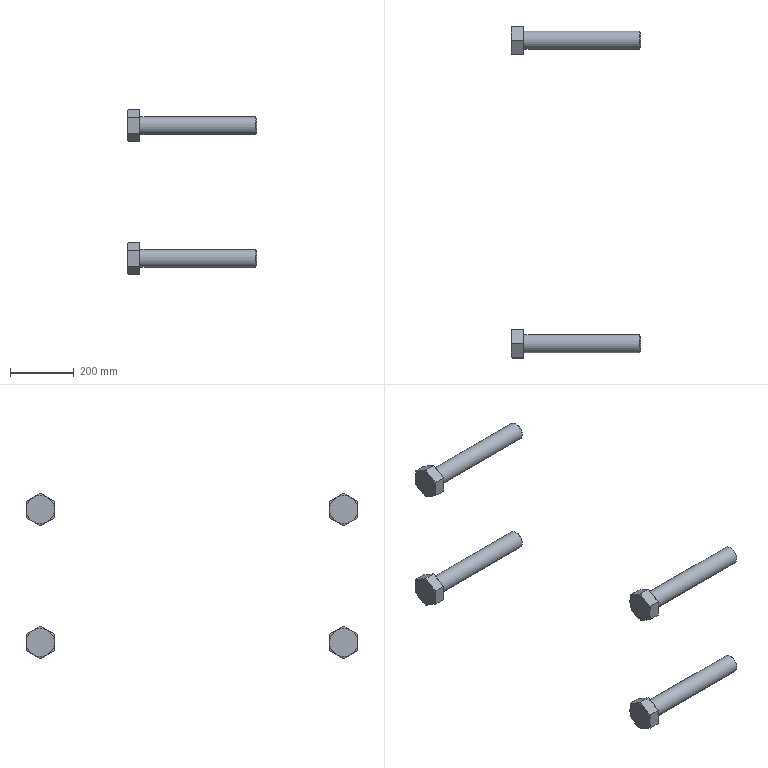Part | NX | features 3.SLDPRT 2, Delete Body 1, LINKED_BODY 1, SCALE 1 | 4 solids | 96 faces | box 405.45 x 1039 x 518.419 mm | volume 4693711 mm3 | plane 60 | cone 32 | cylinder 4 | commonest cylinder face diameters 56.25 x4